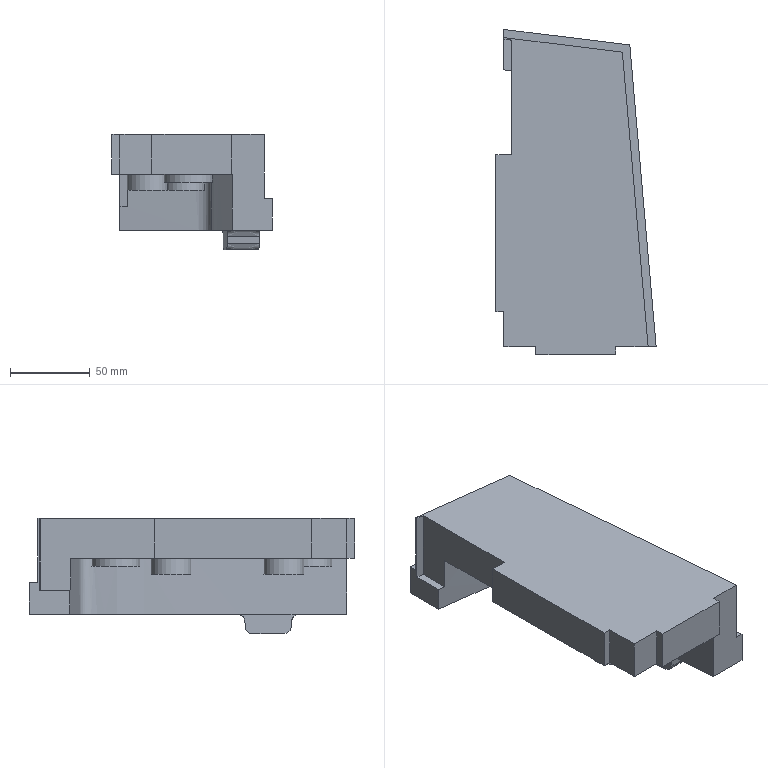Part | NX | features solid 2 | 1 solid | 39 faces | box 100.2 x 203.273 x 72 mm | volume 607336 mm3 | plane 22 | spline 13 | cylinder 4 | commonest cylinder face diameters 25 x2 30 x2